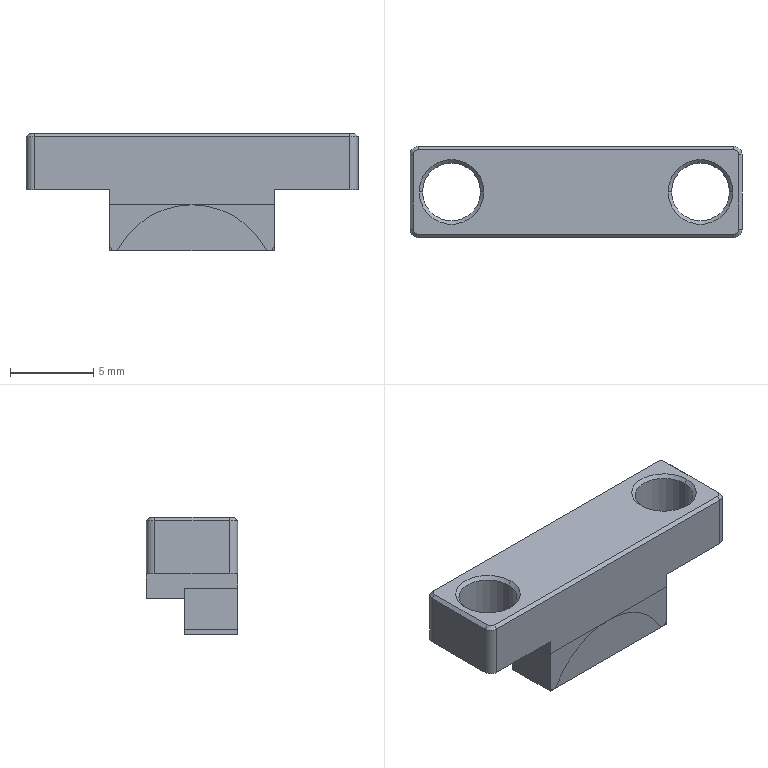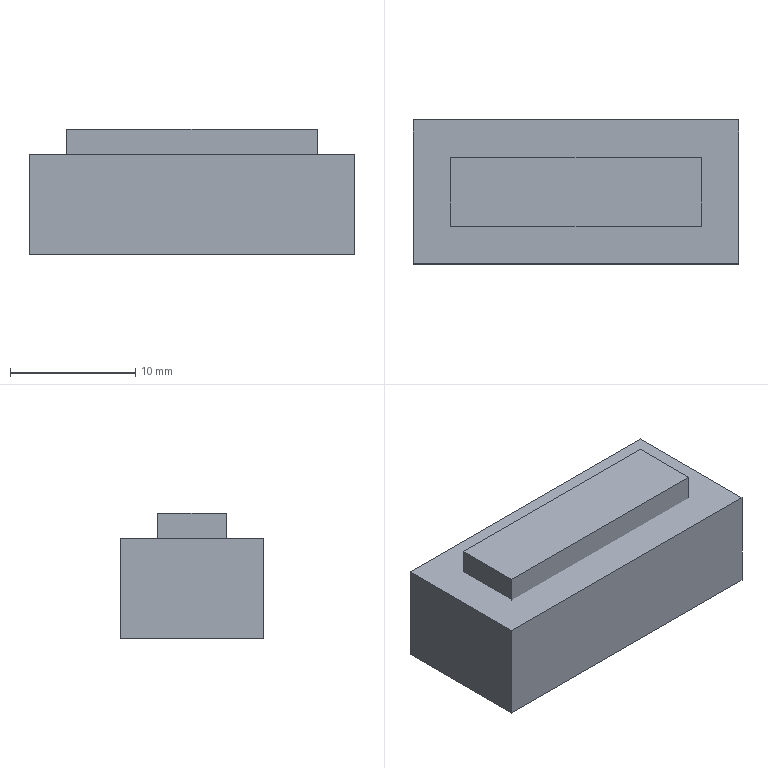CAM job | NX | 3+2 milling, drilling | part box 20 x 5.5 x 7.057 mm | stock box 26 x 11.5 x 10.057 mm
Tools:
number,name,description,diameter,corner_radius,flute_length,length,flutes
3,D63,Milling Tool-5 Parameters,63.0,0.0,50.0,75.0,2
1,D6A45,Milling Tool-5 Parameters,6.0,0.0,3.0,3.0,2
11,3.5ZT,Drilling Tool,3.5,0.0,35.0,50.0,2
16,D6JING,Milling Tool-5 Parameters,6.0,0.0,50.0,75.0,2
12,D2A45,Milling Tool-5 Parameters,2.0,0.0,1.0,1.0,2
17,D4,Milling Tool-5 Parameters,4.0,0.0,50.0,75.0,2
Operations:
program,operation,operation_type,tool,method,geometry_group,spindle_rpm,surface_speed,feed_per_tooth,feed_cut,feed_plunge,cut_length_mm,path_length_mm,cut_time_min,machine_time_min
1,FLOOR_WALL_COPY,VolumeBased25DMillingOperation,D63,METHOD,A,6500.0,1286.0,0.0962,1250.0,100.0,94.998,148.998,0.076,0.0814
1,DRILLING_COPY_1,Operation,D6A45,METHOD,A,5000.0,94.0,0.025,250.0,0.0,9.9,98.097,0.0396,0.0484
1,DRILLING_COPY_1_COPY,Operation,3.5ZT,METHOD,A,2000.0,20.0,0.0625,250.0,0.0,17.903,114.103,0.0716,0.0812
1,ADAPTIVE_MILLING_COPY,CavityMilling,D6JING,METHOD,A,9500.0,179.0,0.1579,3000.0,1000.0,572.254,642.368,0.1914,0.1984
1,ZLEVEL_PROFILE_1_COPY,ZLevelMilling,D6JING,METHOD,A,9500.0,298.0,0.0526,1000.0,100.0,72.879,144.992,0.0729,0.0801
1,11_COPY_COPY,ZLevelMilling,D6A45,METHOD,A,9500.0,179.0,0.0526,1000.0,100.0,64.292,120.292,0.0643,0.0699
2,FLOOR_WALL_COPY_COPY,VolumeBased25DMillingOperation,D63,METHOD,B,6500.0,1286.0,0.0962,1250.0,100.0,284.994,618.99,0.228,0.2614
2,FLOOR_WALL,VolumeBased25DMillingOperation,D6JING,METHOD,B,9500.0,179.0,0.1316,2500.0,1000.0,699.741,975.3,0.3046,0.3322
2,FLOOR_WALL_COPY_1,VolumeBased25DMillingOperation,D6JING,METHOD,B,9500.0,179.0,0.0526,1000.0,1000.0,143.252,429.291,0.1433,0.1728
2,11_COPY_COPY_COPY,ZLevelMilling,D2A45,METHOD,B,9500.0,179.0,0.0526,1000.0,100.0,21.603,80.916,0.0216,0.0275
2,11_COPY_COPY_COPY_COPY,ZLevelMilling,D2A45,METHOD,B,9500.0,179.0,0.0526,1000.0,100.0,75.474,355.531,0.0755,0.1035
3,ZLEVEL_PROFILE_1_COPY_COPY_COPY,ZLevelMilling,D4,METHOD,C,9500.0,298.0,0.1053,2000.0,100.0,161.48,227.88,0.0807,0.0874
3,ZLEVEL_PROFILE_1_COPY_COPY,ZLevelMilling,D4,METHOD,C,9500.0,298.0,0.0526,1000.0,100.0,21.871,86.271,0.0219,0.0283
3,PLANAR_MILL,PlanarMilling,D6A45,METHOD,C,9500.0,179.0,0.0658,1250.0,100.0,67.158,126.158,0.0537,0.0596